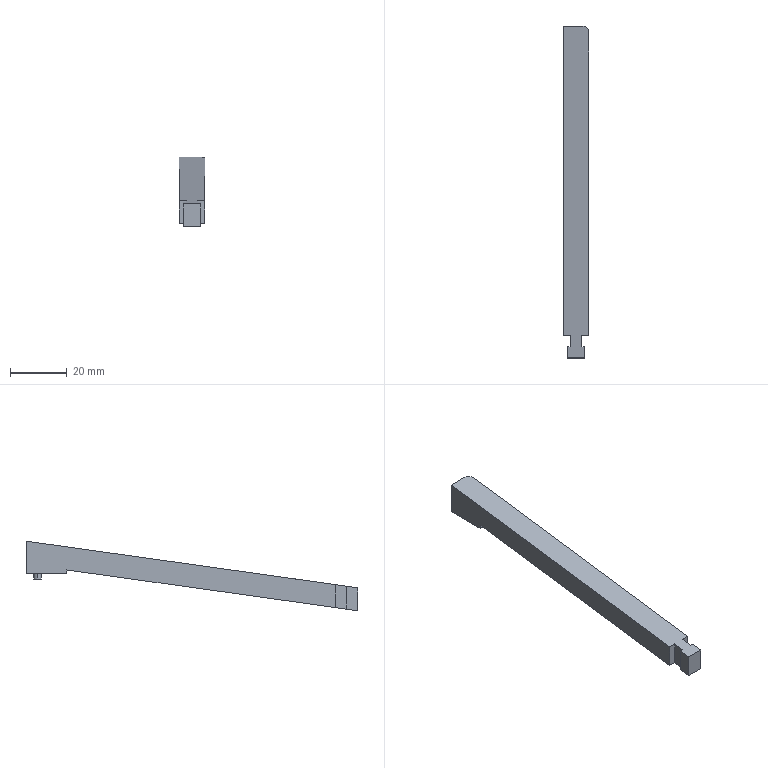Part | STEP file | 1 solid | 24 faces | box 9 x 116.693 x 24.479 mm | volume 8518 mm3 | plane 20 | cylinder 4 | commonest cylinder face diameters 2.513 x2 2.01 x1 4.02 x1